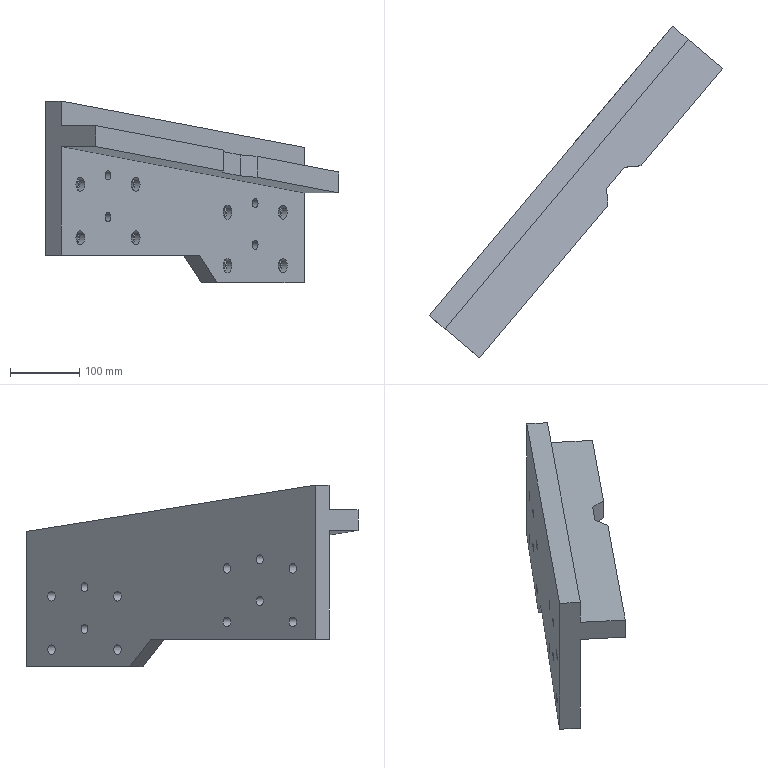Part | NX | features solid 2 | 1 solid | 44 faces | box 423.093 x 478.559 x 262.18 mm | volume 4319267 mm3 | plane 24 | cylinder 20 | commonest cylinder face diameters 14 x8 20 x8 13 x4
STEP:
#1=CARTESIAN_POINT('',(-445.328,317.148,-17.493));
#2=VERTEX_POINT('',#1);
#3=CARTESIAN_POINT('',(-327.504,457.565,-40.));
#4=VERTEX_POINT('',#3);
#5=CARTESIAN_POINT('',(-249.072,551.037,-54.982));
#6=DIRECTION('',(-0.638,-0.7603,0.1219));
#7=VECTOR('',#6,1000.);
#8=LINE('',#5,#7);
#9=EDGE_CURVE('',#2,#4,#8,.F.);
#10=ORIENTED_EDGE('',*,*,#9,.F.);
#11=CARTESIAN_POINT('',(-445.328,317.148,-47.719));
#12=VERTEX_POINT('',#11);
#13=CARTESIAN_POINT('',(-445.328,317.148,-55.974));
#14=DIRECTION('',(0.,0.,-1.));
#15=VECTOR('',#14,1000.);
#16=LINE('',#13,#15);
#17=EDGE_CURVE('',#2,#12,#16,.T.);
#18=ORIENTED_EDGE('',*,*,#17,.T.);
#19=CARTESIAN_POINT('',(-327.504,457.565,-70.225));
#20=VERTEX_POINT('',#19);
#21=CARTESIAN_POINT('',(-281.119,512.845,-79.086));
#22=DIRECTION('',(0.638,0.7603,-0.1219));
#23=VECTOR('',#22,1000.);
#24=LINE('',#21,#23);
#25=EDGE_CURVE('',#12,#20,#24,.T.);
#26=ORIENTED_EDGE('',*,*,#25,.T.);
#27=CARTESIAN_POINT('',(-327.504,457.565,-15.974));
#28=DIRECTION('',(0.,0.,1.));
#29=VECTOR('',#28,1000.);
#30=LINE('',#27,#29);
#31=EDGE_CURVE('',#4,#20,#30,.F.);
#32=ORIENTED_EDGE('',*,*,#31,.F.);
#33=EDGE_LOOP('',(#10,#18,#26,#32));
#34=FACE_BOUND('',#33,.T.);
#35=CARTESIAN_POINT('',(-279.295,515.019,-55.974));
#36=DIRECTION('',(-0.766,0.6428,0.));
#37=DIRECTION('',(-0.6428,-0.766,0.));
#38=AXIS2_PLACEMENT_3D('',#35,#36,#37);
#39=PLANE('',#38);
#40=ADVANCED_FACE('',(#34),#39,.F.);
#41=CARTESIAN_POINT('',(-494.284,359.927,-98.));
#42=VERTEX_POINT('',#41);
#43=CARTESIAN_POINT('',(-487.856,367.587,-98.));
#44=DIRECTION('',(-0.766,0.6428,0.));
#45=DIRECTION('',(-0.6428,-0.766,0.));
#46=AXIS2_PLACEMENT_3D('',#43,#44,#45);
#47=CIRCLE('',#46,10.);
#48=EDGE_CURVE('',#42,#42,#47,.F.);
#49=ORIENTED_EDGE('',*,*,#48,.F.);
#50=EDGE_LOOP('',(#49));
#51=FACE_BOUND('',#50,.T.);
#52=CARTESIAN_POINT('',(-494.284,359.927,-175.));
#53=VERTEX_POINT('',#52);
#54=CARTESIAN_POINT('',(-487.856,367.587,-175.));
#55=DIRECTION('',(-0.766,0.6428,0.));
#56=DIRECTION('',(-0.6428,-0.766,0.));
#57=AXIS2_PLACEMENT_3D('',#54,#55,#56);
#58=CIRCLE('',#57,10.);
#59=EDGE_CURVE('',#53,#53,#58,.F.);
#60=ORIENTED_EDGE('',*,*,#59,.F.);
#61=EDGE_LOOP('',(#60));
#62=FACE_BOUND('',#61,.T.);
#63=CARTESIAN_POINT('',(-626.698,202.121,-135.));
#64=VERTEX_POINT('',#63);
#65=CARTESIAN_POINT('',(-620.271,209.782,-135.));
#66=DIRECTION('',(-0.766,0.6428,0.));
#67=DIRECTION('',(-0.6428,-0.766,0.));
#68=AXIS2_PLACEMENT_3D('',#65,#66,#67);
#69=CIRCLE('',#68,10.);
#70=EDGE_CURVE('',#64,#64,#69,.F.);
#71=ORIENTED_EDGE('',*,*,#70,.F.);
#72=EDGE_LOOP('',(#71));
#73=FACE_BOUND('',#72,.T.);
#74=CARTESIAN_POINT('',(-706.404,107.132,-58.));
#75=VERTEX_POINT('',#74);
#76=CARTESIAN_POINT('',(-699.976,114.792,-58.));
#77=DIRECTION('',(-0.766,0.6428,0.));
#78=DIRECTION('',(-0.6428,-0.766,0.));
#79=AXIS2_PLACEMENT_3D('',#76,#77,#78);
#80=CIRCLE('',#79,10.);
#81=EDGE_CURVE('',#75,#75,#80,.F.);
#82=ORIENTED_EDGE('',*,*,#81,.F.);
#83=EDGE_LOOP('',(#82));
#84=FACE_BOUND('',#83,.T.);
#85=CARTESIAN_POINT('',(-727.616,81.852,-160.));
#86=VERTEX_POINT('',#85);
#87=CARTESIAN_POINT('',(-528.352,319.326,-160.));
#88=VERTEX_POINT('',#87);
#89=CARTESIAN_POINT('',(-727.616,81.852,-160.));
#90=DIRECTION('',(0.6428,0.766,0.));
#91=VECTOR('',#90,1000.);
#92=LINE('',#89,#91);
#93=EDGE_CURVE('',#86,#88,#92,.T.);
#94=ORIENTED_EDGE('',*,*,#93,.T.);
#95=CARTESIAN_POINT('',(-502.64,349.968,-200.));
#96=VERTEX_POINT('',#95);
#97=CARTESIAN_POINT('',(-475.009,382.898,-242.987));
#98=DIRECTION('',(0.4545,0.5417,-0.7071));
#99=VECTOR('',#98,1000.);
#100=LINE('',#97,#99);
#101=EDGE_CURVE('',#88,#96,#100,.T.);
#102=ORIENTED_EDGE('',*,*,#101,.T.);
#103=CARTESIAN_POINT('',(-377.297,499.347,-200.));
#104=VERTEX_POINT('',#103);
#105=CARTESIAN_POINT('',(-329.088,556.8,-200.));
#106=DIRECTION('',(-0.6428,-0.766,0.));
#107=VECTOR('',#106,1000.);
#108=LINE('',#105,#107);
#109=EDGE_CURVE('',#96,#104,#108,.F.);
#110=ORIENTED_EDGE('',*,*,#109,.T.);
#111=CARTESIAN_POINT('',(-377.297,499.347,-70.225));
#112=VERTEX_POINT('',#111);
#113=CARTESIAN_POINT('',(-377.297,499.347,-15.974));
#114=DIRECTION('',(0.,0.,1.));
#115=VECTOR('',#114,1000.);
#116=LINE('',#113,#115);
#117=EDGE_CURVE('',#112,#104,#116,.F.);
#118=ORIENTED_EDGE('',*,*,#117,.F.);
#119=CARTESIAN_POINT('',(-727.616,81.852,-3.308));
#120=VERTEX_POINT('',#119);
#121=CARTESIAN_POINT('',(-553.34,289.547,-36.598));
#122=DIRECTION('',(0.638,0.7603,-0.1219));
#123=VECTOR('',#122,1000.);
#124=LINE('',#121,#123);
#125=EDGE_CURVE('',#120,#112,#124,.T.);
#126=ORIENTED_EDGE('',*,*,#125,.F.);
#127=CARTESIAN_POINT('',(-727.616,81.852,-70.036));
#128=DIRECTION('',(0.,0.,-1.));
#129=VECTOR('',#128,1000.);
#130=LINE('',#127,#129);
#131=EDGE_CURVE('',#86,#120,#130,.F.);
#132=ORIENTED_EDGE('',*,*,#131,.F.);
#133=EDGE_LOOP('',(#94,#102,#110,#118,#126,#132));
#134=FACE_BOUND('',#133,.T.);
#135=CARTESIAN_POINT('',(-664.302,157.308,-105.));
#136=VERTEX_POINT('',#135);
#137=CARTESIAN_POINT('',(-660.123,162.287,-105.));
#138=DIRECTION('',(-0.766,0.6428,0.));
#139=DIRECTION('',(-0.6428,-0.766,0.));
#140=AXIS2_PLACEMENT_3D('',#137,#138,#139);
#141=CIRCLE('',#140,6.5);
#142=EDGE_CURVE('',#136,#136,#141,.T.);
#143=ORIENTED_EDGE('',*,*,#142,.T.);
#144=EDGE_LOOP('',(#143));
#145=FACE_BOUND('',#144,.T.);
#146=CARTESIAN_POINT('',(-664.302,157.308,-45.));
#147=VERTEX_POINT('',#146);
#148=CARTESIAN_POINT('',(-660.123,162.287,-45.));
#149=DIRECTION('',(-0.766,0.6428,0.));
#150=DIRECTION('',(-0.6428,-0.766,0.));
#151=AXIS2_PLACEMENT_3D('',#148,#149,#150);
#152=CIRCLE('',#151,6.5);
#153=EDGE_CURVE('',#147,#147,#152,.T.);
#154=ORIENTED_EDGE('',*,*,#153,.T.);
#155=EDGE_LOOP('',(#154));
#156=FACE_BOUND('',#155,.T.);
#157=CARTESIAN_POINT('',(-452.182,410.102,-145.));
#158=VERTEX_POINT('',#157);
#159=CARTESIAN_POINT('',(-448.003,415.082,-145.));
#160=DIRECTION('',(-0.766,0.6428,0.));
#161=DIRECTION('',(-0.6428,-0.766,0.));
#162=AXIS2_PLACEMENT_3D('',#159,#160,#161);
#163=CIRCLE('',#162,6.5);
#164=EDGE_CURVE('',#158,#158,#163,.T.);
#165=ORIENTED_EDGE('',*,*,#164,.T.);
#166=EDGE_LOOP('',(#165));
#167=FACE_BOUND('',#166,.T.);
#168=CARTESIAN_POINT('',(-452.182,410.102,-85.));
#169=VERTEX_POINT('',#168);
#170=CARTESIAN_POINT('',(-448.003,415.082,-85.));
#171=DIRECTION('',(-0.766,0.6428,0.));
#172=DIRECTION('',(-0.6428,-0.766,0.));
#173=AXIS2_PLACEMENT_3D('',#170,#171,#172);
#174=CIRCLE('',#173,6.5);
#175=EDGE_CURVE('',#169,#169,#174,.T.);
#176=ORIENTED_EDGE('',*,*,#175,.T.);
#177=EDGE_LOOP('',(#176));
#178=FACE_BOUND('',#177,.T.);
#179=CARTESIAN_POINT('',(-706.404,107.132,-135.));
#180=VERTEX_POINT('',#179);
#181=CARTESIAN_POINT('',(-699.976,114.792,-135.));
#182=DIRECTION('',(-0.766,0.6428,0.));
#183=DIRECTION('',(-0.6428,-0.766,0.));
#184=AXIS2_PLACEMENT_3D('',#181,#182,#183);
#185=CIRCLE('',#184,10.);
#186=EDGE_CURVE('',#180,#180,#185,.F.);
#187=ORIENTED_EDGE('',*,*,#186,.F.);
#188=EDGE_LOOP('',(#187));
#189=FACE_BOUND('',#188,.T.);
#190=CARTESIAN_POINT('',(-626.698,202.121,-58.));
#191=VERTEX_POINT('',#190);
#192=CARTESIAN_POINT('',(-620.271,209.782,-58.));
#193=DIRECTION('',(-0.766,0.6428,0.));
#194=DIRECTION('',(-0.6428,-0.766,0.));
#195=AXIS2_PLACEMENT_3D('',#192,#193,#194);
#196=CIRCLE('',#195,10.);
#197=EDGE_CURVE('',#191,#191,#196,.F.);
#198=ORIENTED_EDGE('',*,*,#197,.F.);
#199=EDGE_LOOP('',(#198));
#200=FACE_BOUND('',#199,.T.);
#201=CARTESIAN_POINT('',(-414.579,454.916,-175.));
#202=VERTEX_POINT('',#201);
#203=CARTESIAN_POINT('',(-408.151,462.577,-175.));
#204=DIRECTION('',(-0.766,0.6428,0.));
#205=DIRECTION('',(-0.6428,-0.766,0.));
#206=AXIS2_PLACEMENT_3D('',#203,#204,#205);
#207=CIRCLE('',#206,10.);
#208=EDGE_CURVE('',#202,#202,#207,.F.);
#209=ORIENTED_EDGE('',*,*,#208,.F.);
#210=EDGE_LOOP('',(#209));
#211=FACE_BOUND('',#210,.T.);
#212=CARTESIAN_POINT('',(-414.579,454.916,-98.));
#213=VERTEX_POINT('',#212);
#214=CARTESIAN_POINT('',(-408.151,462.577,-98.));
#215=DIRECTION('',(-0.766,0.6428,0.));
#216=DIRECTION('',(-0.6428,-0.766,0.));
#217=AXIS2_PLACEMENT_3D('',#214,#215,#216);
#218=CIRCLE('',#217,10.);
#219=EDGE_CURVE('',#213,#213,#218,.F.);
#220=ORIENTED_EDGE('',*,*,#219,.F.);
#221=EDGE_LOOP('',(#220));
#222=FACE_BOUND('',#221,.T.);
#223=CARTESIAN_POINT('',(-329.088,556.8,-15.974));
#224=DIRECTION('',(-0.766,0.6428,0.));
#225=DIRECTION('',(-0.6428,-0.766,0.));
#226=AXIS2_PLACEMENT_3D('',#223,#224,#225);
#227=PLANE('',#226);
#228=ADVANCED_FACE('',(#51,#62,#73,#84,#134,#145,#156,#167,#178,#189,#200,#211,#222),#227,.F.);
#229=CARTESIAN_POINT('',(-525.622,369.252,-200.));
#230=VERTEX_POINT('',#229);
#231=CARTESIAN_POINT('',(-400.278,518.63,-200.));
#232=VERTEX_POINT('',#231);
#233=CARTESIAN_POINT('',(-352.069,576.084,-200.));
#234=DIRECTION('',(-0.6428,-0.766,0.));
#235=VECTOR('',#234,1000.);
#236=LINE('',#233,#235);
#237=EDGE_CURVE('',#230,#232,#236,.F.);
#238=ORIENTED_EDGE('',*,*,#237,.F.);
#239=CARTESIAN_POINT('',(-551.333,338.61,-160.));
#240=VERTEX_POINT('',#239);
#241=CARTESIAN_POINT('',(-551.333,338.61,-160.));
#242=DIRECTION('',(-0.4545,-0.5417,0.7071));
#243=VECTOR('',#242,1000.);
#244=LINE('',#241,#243);
#245=EDGE_CURVE('',#230,#240,#244,.T.);
#246=ORIENTED_EDGE('',*,*,#245,.T.);
#247=CARTESIAN_POINT('',(-750.597,101.136,-160.));
#248=VERTEX_POINT('',#247);
#249=CARTESIAN_POINT('',(-750.597,101.136,-160.));
#250=DIRECTION('',(0.6428,0.766,0.));
#251=VECTOR('',#250,1000.);
#252=LINE('',#249,#251);
#253=EDGE_CURVE('',#248,#240,#252,.T.);
#254=ORIENTED_EDGE('',*,*,#253,.F.);
#255=CARTESIAN_POINT('',(-750.597,101.136,62.18));
#256=VERTEX_POINT('',#255);
#257=CARTESIAN_POINT('',(-750.597,101.136,-15.974));
#258=DIRECTION('',(0.,0.,1.));
#259=VECTOR('',#258,1000.);
#260=LINE('',#257,#259);
#261=EDGE_CURVE('',#256,#248,#260,.F.);
#262=ORIENTED_EDGE('',*,*,#261,.F.);
#263=CARTESIAN_POINT('',(-400.278,518.63,-4.737));
#264=VERTEX_POINT('',#263);
#265=CARTESIAN_POINT('',(-319.104,615.369,-20.243));
#266=DIRECTION('',(-0.638,-0.7603,0.1219));
#267=VECTOR('',#266,1000.);
#268=LINE('',#265,#267);
#269=EDGE_CURVE('',#256,#264,#268,.F.);
#270=ORIENTED_EDGE('',*,*,#269,.T.);
#271=CARTESIAN_POINT('',(-400.278,518.63,-15.974));
#272=DIRECTION('',(0.,0.,1.));
#273=VECTOR('',#272,1000.);
#274=LINE('',#271,#273);
#275=EDGE_CURVE('',#264,#232,#274,.F.);
#276=ORIENTED_EDGE('',*,*,#275,.T.);
#277=EDGE_LOOP('',(#238,#246,#254,#262,#270,#276));
#278=FACE_BOUND('',#277,.T.);
#279=CARTESIAN_POINT('',(-647.751,223.703,-58.));
#280=VERTEX_POINT('',#279);
#281=CARTESIAN_POINT('',(-643.252,229.065,-58.));
#282=DIRECTION('',(-0.766,0.6428,0.));
#283=DIRECTION('',(-0.6428,-0.766,0.));
#284=AXIS2_PLACEMENT_3D('',#281,#282,#283);
#285=CIRCLE('',#284,7.);
#286=EDGE_CURVE('',#280,#280,#285,.F.);
#287=ORIENTED_EDGE('',*,*,#286,.T.);
#288=EDGE_LOOP('',(#287));
#289=FACE_BOUND('',#288,.T.);
#290=CARTESIAN_POINT('',(-687.283,176.591,-45.));
#291=VERTEX_POINT('',#290);
#292=CARTESIAN_POINT('',(-683.105,181.571,-45.));
#293=DIRECTION('',(-0.766,0.6428,0.));
#294=DIRECTION('',(-0.6428,-0.766,0.));
#295=AXIS2_PLACEMENT_3D('',#292,#293,#294);
#296=CIRCLE('',#295,6.5);
#297=EDGE_CURVE('',#291,#291,#296,.T.);
#298=ORIENTED_EDGE('',*,*,#297,.F.);
#299=EDGE_LOOP('',(#298));
#300=FACE_BOUND('',#299,.T.);
#301=CARTESIAN_POINT('',(-647.751,223.703,-135.));
#302=VERTEX_POINT('',#301);
#303=CARTESIAN_POINT('',(-643.252,229.065,-135.));
#304=DIRECTION('',(-0.766,0.6428,0.));
#305=DIRECTION('',(-0.6428,-0.766,0.));
#306=AXIS2_PLACEMENT_3D('',#303,#304,#305);
#307=CIRCLE('',#306,7.);
#308=EDGE_CURVE('',#302,#302,#307,.F.);
#309=ORIENTED_EDGE('',*,*,#308,.T.);
#310=EDGE_LOOP('',(#309));
#311=FACE_BOUND('',#310,.T.);
#312=CARTESIAN_POINT('',(-687.283,176.591,-105.));
#313=VERTEX_POINT('',#312);
#314=CARTESIAN_POINT('',(-683.105,181.571,-105.));
#315=DIRECTION('',(-0.766,0.6428,0.));
#316=DIRECTION('',(-0.6428,-0.766,0.));
#317=AXIS2_PLACEMENT_3D('',#314,#315,#316);
#318=CIRCLE('',#317,6.5);
#319=EDGE_CURVE('',#313,#313,#318,.T.);
#320=ORIENTED_EDGE('',*,*,#319,.F.);
#321=EDGE_LOOP('',(#320));
#322=FACE_BOUND('',#321,.T.);
#323=CARTESIAN_POINT('',(-727.457,128.714,-135.));
#324=VERTEX_POINT('',#323);
#325=CARTESIAN_POINT('',(-722.958,134.076,-135.));
#326=DIRECTION('',(-0.766,0.6428,0.));
#327=DIRECTION('',(-0.6428,-0.766,0.));
#328=AXIS2_PLACEMENT_3D('',#325,#326,#327);
#329=CIRCLE('',#328,7.);
#330=EDGE_CURVE('',#324,#324,#329,.F.);
#331=ORIENTED_EDGE('',*,*,#330,.T.);
#332=EDGE_LOOP('',(#331));
#333=FACE_BOUND('',#332,.T.);
#334=CARTESIAN_POINT('',(-727.457,128.714,-58.));
#335=VERTEX_POINT('',#334);
#336=CARTESIAN_POINT('',(-722.958,134.076,-58.));
#337=DIRECTION('',(-0.766,0.6428,0.));
#338=DIRECTION('',(-0.6428,-0.766,0.));
#339=AXIS2_PLACEMENT_3D('',#336,#337,#338);
#340=CIRCLE('',#339,7.);
#341=EDGE_CURVE('',#335,#335,#340,.F.);
#342=ORIENTED_EDGE('',*,*,#341,.T.);
#343=EDGE_LOOP('',(#342));
#344=FACE_BOUND('',#343,.T.);
#345=CARTESIAN_POINT('',(-435.631,476.498,-98.));
#346=VERTEX_POINT('',#345);
#347=CARTESIAN_POINT('',(-431.132,481.86,-98.));
#348=DIRECTION('',(-0.766,0.6428,0.));
#349=DIRECTION('',(-0.6428,-0.766,0.));
#350=AXIS2_PLACEMENT_3D('',#347,#348,#349);
#351=CIRCLE('',#350,7.);
#352=EDGE_CURVE('',#346,#346,#351,.F.);
#353=ORIENTED_EDGE('',*,*,#352,.T.);
#354=EDGE_LOOP('',(#353));
#355=FACE_BOUND('',#354,.T.);
#356=CARTESIAN_POINT('',(-475.163,429.386,-85.));
#357=VERTEX_POINT('',#356);
#358=CARTESIAN_POINT('',(-470.985,434.365,-85.));
#359=DIRECTION('',(-0.766,0.6428,0.));
#360=DIRECTION('',(-0.6428,-0.766,0.));
#361=AXIS2_PLACEMENT_3D('',#358,#359,#360);
#362=CIRCLE('',#361,6.5);
#363=EDGE_CURVE('',#357,#357,#362,.T.);
#364=ORIENTED_EDGE('',*,*,#363,.F.);
#365=EDGE_LOOP('',(#364));
#366=FACE_BOUND('',#365,.T.);
#367=CARTESIAN_POINT('',(-435.631,476.498,-175.));
#368=VERTEX_POINT('',#367);
#369=CARTESIAN_POINT('',(-431.132,481.86,-175.));
#370=DIRECTION('',(-0.766,0.6428,0.));
#371=DIRECTION('',(-0.6428,-0.766,0.));
#372=AXIS2_PLACEMENT_3D('',#369,#370,#371);
#373=CIRCLE('',#372,7.);
#374=EDGE_CURVE('',#368,#368,#373,.F.);
#375=ORIENTED_EDGE('',*,*,#374,.T.);
#376=EDGE_LOOP('',(#375));
#377=FACE_BOUND('',#376,.T.);
#378=CARTESIAN_POINT('',(-475.163,429.386,-145.));
#379=VERTEX_POINT('',#378);
#380=CARTESIAN_POINT('',(-470.985,434.365,-145.));
#381=DIRECTION('',(-0.766,0.6428,0.));
#382=DIRECTION('',(-0.6428,-0.766,0.));
#383=AXIS2_PLACEMENT_3D('',#380,#381,#382);
#384=CIRCLE('',#383,6.5);
#385=EDGE_CURVE('',#379,#379,#384,.T.);
#386=ORIENTED_EDGE('',*,*,#385,.F.);
#387=EDGE_LOOP('',(#386));
#388=FACE_BOUND('',#387,.T.);
#389=CARTESIAN_POINT('',(-515.337,381.508,-175.));
#390=VERTEX_POINT('',#389);
#391=CARTESIAN_POINT('',(-510.838,386.871,-175.));
#392=DIRECTION('',(-0.766,0.6428,0.));
#393=DIRECTION('',(-0.6428,-0.766,0.));
#394=AXIS2_PLACEMENT_3D('',#391,#392,#393);
#395=CIRCLE('',#394,7.);
#396=EDGE_CURVE('',#390,#390,#395,.F.);
#397=ORIENTED_EDGE('',*,*,#396,.T.);
#398=EDGE_LOOP('',(#397));
#399=FACE_BOUND('',#398,.T.);
#400=CARTESIAN_POINT('',(-515.337,381.508,-98.));
#401=VERTEX_POINT('',#400);
#402=CARTESIAN_POINT('',(-510.838,386.871,-98.));
#403=DIRECTION('',(-0.766,0.6428,0.));
#404=DIRECTION('',(-0.6428,-0.766,0.));
#405=AXIS2_PLACEMENT_3D('',#402,#403,#404);
#406=CIRCLE('',#405,7.);
#407=EDGE_CURVE('',#401,#401,#406,.F.);
#408=ORIENTED_EDGE('',*,*,#407,.T.);
#409=EDGE_LOOP('',(#408));
#410=FACE_BOUND('',#409,.T.);
#411=CARTESIAN_POINT('',(-352.069,576.084,-15.974));
#412=DIRECTION('',(-0.766,0.6428,0.));
#413=DIRECTION('',(-0.6428,-0.766,0.));
#414=AXIS2_PLACEMENT_3D('',#411,#412,#413);
#415=PLANE('',#414);
#416=ADVANCED_FACE('',(#278,#289,#300,#311,#322,#333,#344,#355,#366,#377,#388,#399,#410),#415,.T.);
#417=ORIENTED_EDGE('',*,*,#25,.F.);
#418=CARTESIAN_POINT('',(-469.331,315.048,-45.627));
#419=VERTEX_POINT('',#418);
#420=CARTESIAN_POINT('',(-555.051,307.548,-38.156));
#421=DIRECTION('',(-0.9925,-0.08683,0.0865));
#422=VECTOR('',#421,1000.);
#423=LINE('',#420,#422);
#424=EDGE_CURVE('',#12,#419,#423,.T.);
#425=ORIENTED_EDGE('',*,*,#424,.T.);
#426=CARTESIAN_POINT('',(-495.043,284.406,-40.715));
#427=VERTEX_POINT('',#426);
#428=CARTESIAN_POINT('',(-516.599,258.717,-36.598));
#429=DIRECTION('',(0.638,0.7603,-0.1219));
#430=VECTOR('',#429,1000.);
#431=LINE('',#428,#430);
#432=EDGE_CURVE('',#427,#419,#431,.T.);
#433=ORIENTED_EDGE('',*,*,#432,.F.);
#434=CARTESIAN_POINT('',(-492.943,260.403,-38.623));
#435=VERTEX_POINT('',#434);
#436=CARTESIAN_POINT('',(-495.895,294.14,-41.564));
#437=DIRECTION('',(0.08683,-0.9925,0.0865));
#438=VECTOR('',#437,1000.);
#439=LINE('',#436,#438);
#440=EDGE_CURVE('',#427,#435,#439,.T.);
#441=ORIENTED_EDGE('',*,*,#440,.T.);
#442=CARTESIAN_POINT('',(-677.823,40.071,-3.308));
#443=VERTEX_POINT('',#442);
#444=CARTESIAN_POINT('',(-281.119,512.845,-79.086));
#445=DIRECTION('',(0.638,0.7603,-0.1219));
#446=VECTOR('',#445,1000.);
#447=LINE('',#444,#446);
#448=EDGE_CURVE('',#443,#435,#447,.T.);
#449=ORIENTED_EDGE('',*,*,#448,.F.);
#450=CARTESIAN_POINT('',(-727.616,81.852,-3.308));
#451=DIRECTION('',(0.766,-0.6428,0.));
#452=VECTOR('',#451,1000.);
#453=LINE('',#450,#452);
#454=EDGE_CURVE('',#443,#120,#453,.F.);
#455=ORIENTED_EDGE('',*,*,#454,.T.);
#456=ORIENTED_EDGE('',*,*,#125,.T.);
#457=CARTESIAN_POINT('',(-377.297,499.347,-70.225));
#458=DIRECTION('',(0.766,-0.6428,0.));
#459=VECTOR('',#458,1000.);
#460=LINE('',#457,#459);
#461=EDGE_CURVE('',#20,#112,#460,.F.);
#462=ORIENTED_EDGE('',*,*,#461,.F.);
#463=EDGE_LOOP('',(#417,#425,#433,#441,#449,#455,#456,#462));
#464=FACE_BOUND('',#463,.T.);
#465=CARTESIAN_POINT('',(-553.34,289.547,-36.598));
#466=DIRECTION('',(0.07834,0.09336,0.9925));
#467=DIRECTION('',(0.638,0.7603,-0.1219));
#468=AXIS2_PLACEMENT_3D('',#465,#466,#467);
#469=PLANE('',#468);
#470=ADVANCED_FACE('',(#464),#469,.F.);
#471=CARTESIAN_POINT('',(-727.616,81.852,26.918));
#472=VERTEX_POINT('',#471);
#473=CARTESIAN_POINT('',(-377.297,499.347,-40.));
#474=VERTEX_POINT('',#473);
#475=CARTESIAN_POINT('',(-298.865,592.818,-54.982));
#476=DIRECTION('',(-0.638,-0.7603,0.1219));
#477=VECTOR('',#476,1000.);
#478=LINE('',#475,#477);
#479=EDGE_CURVE('',#472,#474,#478,.F.);
#480=ORIENTED_EDGE('',*,*,#479,.T.);
#481=CARTESIAN_POINT('',(-377.297,499.347,-4.737));
#482=VERTEX_POINT('',#481);
#483=CARTESIAN_POINT('',(-377.297,499.347,-15.974));
#484=DIRECTION('',(0.,0.,1.));
#485=VECTOR('',#484,1000.);
#486=LINE('',#483,#485);
#487=EDGE_CURVE('',#482,#474,#486,.F.);
#488=ORIENTED_EDGE('',*,*,#487,.F.);
#489=CARTESIAN_POINT('',(-727.616,81.852,62.18));
#490=VERTEX_POINT('',#489);
#491=CARTESIAN_POINT('',(-296.123,596.086,-20.243));
#492=DIRECTION('',(-0.638,-0.7603,0.1219));
#493=VECTOR('',#492,1000.);
#494=LINE('',#491,#493);
#495=EDGE_CURVE('',#490,#482,#494,.F.);
#496=ORIENTED_EDGE('',*,*,#495,.F.);
#497=CARTESIAN_POINT('',(-727.616,81.852,-15.974));
#498=DIRECTION('',(0.,0.,1.));
#499=VECTOR('',#498,1000.);
#500=LINE('',#497,#499);
#501=EDGE_CURVE('',#490,#472,#500,.F.);
#502=ORIENTED_EDGE('',*,*,#501,.T.);
#503=EDGE_LOOP('',(#480,#488,#496,#502));
#504=FACE_BOUND('',#503,.T.);
#505=CARTESIAN_POINT('',(-329.088,556.8,-15.974));
#506=DIRECTION('',(-0.766,0.6428,0.));
#507=DIRECTION('',(-0.6428,-0.766,0.));
#508=AXIS2_PLACEMENT_3D('',#505,#506,#507);
#509=PLANE('',#508);
#510=ADVANCED_FACE('',(#504),#509,.F.);
#511=ORIENTED_EDGE('',*,*,#495,.T.);
#512=CARTESIAN_POINT('',(-377.297,499.347,-4.737));
#513=DIRECTION('',(-0.766,0.6428,0.));
#514=VECTOR('',#513,1000.);
#515=LINE('',#512,#514);
#516=EDGE_CURVE('',#482,#264,#515,.T.);
#517=ORIENTED_EDGE('',*,*,#516,.T.);
#518=ORIENTED_EDGE('',*,*,#269,.F.);
#519=CARTESIAN_POINT('',(-727.616,81.852,62.18));
#520=DIRECTION('',(-0.766,0.6428,0.));
#521=VECTOR('',#520,1000.);
#522=LINE('',#519,#521);
#523=EDGE_CURVE('',#490,#256,#522,.T.);
#524=ORIENTED_EDGE('',*,*,#523,.F.);
#525=EDGE_LOOP('',(#511,#517,#518,#524));
#526=FACE_BOUND('',#525,.T.);
#527=CARTESIAN_POINT('',(-296.123,596.086,-20.243));
#528=DIRECTION('',(0.07834,0.09336,0.9925));
#529=DIRECTION('',(0.,-0.9956,0.09365));
#530=AXIS2_PLACEMENT_3D('',#527,#528,#529);
#531=PLANE('',#530);
#532=ADVANCED_FACE('',(#526),#531,.T.);
#533=ORIENTED_EDGE('',*,*,#109,.F.);
#534=CARTESIAN_POINT('',(-525.622,369.252,-200.));
#535=DIRECTION('',(0.766,-0.6428,0.));
#536=VECTOR('',#535,1000.);
#537=LINE('',#534,#536);
#538=EDGE_CURVE('',#230,#96,#537,.T.);
#539=ORIENTED_EDGE('',*,*,#538,.F.);
#540=ORIENTED_EDGE('',*,*,#237,.T.);
#541=CARTESIAN_POINT('',(-400.278,518.63,-200.));
#542=DIRECTION('',(-0.766,0.6428,0.));
#543=VECTOR('',#542,1000.);
#544=LINE('',#541,#543);
#545=EDGE_CURVE('',#104,#232,#544,.T.);
#546=ORIENTED_EDGE('',*,*,#545,.F.);
#547=EDGE_LOOP('',(#533,#539,#540,#546));
#548=FACE_BOUND('',#547,.T.);
#549=CARTESIAN_POINT('',(-470.985,434.365,-200.));
#550=DIRECTION('',(0.,0.,-1.));
#551=DIRECTION('',(-0.766,0.6428,0.));
#552=AXIS2_PLACEMENT_3D('',#549,#550,#551);
#553=PLANE('',#552);
#554=ADVANCED_FACE('',(#548),#553,.T.);
#555=ORIENTED_EDGE('',*,*,#461,.T.);
#556=ORIENTED_EDGE('',*,*,#117,.T.);
#557=ORIENTED_EDGE('',*,*,#545,.T.);
#558=ORIENTED_EDGE('',*,*,#275,.F.);
#559=ORIENTED_EDGE('',*,*,#516,.F.);
#560=ORIENTED_EDGE('',*,*,#487,.T.);
#561=CARTESIAN_POINT('',(-377.297,499.347,-40.));
#562=DIRECTION('',(0.766,-0.6428,0.));
#563=VECTOR('',#562,1000.);
#564=LINE('',#561,#563);
#565=EDGE_CURVE('',#474,#4,#564,.T.);
#566=ORIENTED_EDGE('',*,*,#565,.T.);
#567=ORIENTED_EDGE('',*,*,#31,.T.);
#568=EDGE_LOOP('',(#555,#556,#557,#558,#559,#560,#566,#567));
#569=FACE_BOUND('',#568,.T.);
#570=CARTESIAN_POINT('',(-377.297,499.347,-15.974));
#571=DIRECTION('',(0.6428,0.766,0.));
#572=DIRECTION('',(0.,0.,-1.));
#573=AXIS2_PLACEMENT_3D('',#570,#571,#572);
#574=PLANE('',#573);
#575=ADVANCED_FACE('',(#569),#574,.T.);
#576=ORIENTED_EDGE('',*,*,#448,.T.);
#577=CARTESIAN_POINT('',(-492.943,260.403,-8.398));
#578=VERTEX_POINT('',#577);
#579=CARTESIAN_POINT('',(-492.943,260.403,-55.974));
#580=DIRECTION('',(0.,0.,1.));
#581=VECTOR('',#580,1000.);
#582=LINE('',#579,#581);
#583=EDGE_CURVE('',#435,#578,#582,.T.);
#584=ORIENTED_EDGE('',*,*,#583,.T.);
#585=CARTESIAN_POINT('',(-677.823,40.071,26.918));
#586=VERTEX_POINT('',#585);
#587=CARTESIAN_POINT('',(-249.072,551.037,-54.982));
#588=DIRECTION('',(-0.638,-0.7603,0.1219));
#589=VECTOR('',#588,1000.);
#590=LINE('',#587,#589);
#591=EDGE_CURVE('',#586,#578,#590,.F.);
#592=ORIENTED_EDGE('',*,*,#591,.F.);
#593=CARTESIAN_POINT('',(-677.823,40.071,-55.974));
#594=DIRECTION('',(0.,0.,1.));
#595=VECTOR('',#594,1000.);
#596=LINE('',#593,#595);
#597=EDGE_CURVE('',#586,#443,#596,.F.);
#598=ORIENTED_EDGE('',*,*,#597,.T.);
#599=EDGE_LOOP('',(#576,#584,#592,#598));
#600=FACE_BOUND('',#599,.T.);
#601=CARTESIAN_POINT('',(-279.295,515.019,-55.974));
#602=DIRECTION('',(-0.766,0.6428,0.));
#603=DIRECTION('',(-0.6428,-0.766,0.));
#604=AXIS2_PLACEMENT_3D('',#601,#602,#603);
#605=PLANE('',#604);
#606=ADVANCED_FACE('',(#600),#605,.F.);
#607=CARTESIAN_POINT('',(-469.331,315.048,-15.401));
#608=VERTEX_POINT('',#607);
#609=CARTESIAN_POINT('',(-495.043,284.406,-10.49));
#610=VERTEX_POINT('',#609);
#611=CARTESIAN_POINT('',(-262.123,561.989,-54.982));
#612=DIRECTION('',(0.638,0.7603,-0.1219));
#613=VECTOR('',#612,1000.);
#614=LINE('',#611,#613);
#615=EDGE_CURVE('',#608,#610,#614,.F.);
#616=ORIENTED_EDGE('',*,*,#615,.F.);
#617=CARTESIAN_POINT('',(-274.091,332.129,-32.417));
#618=DIRECTION('',(-0.9925,-0.08683,0.0865));
#619=VECTOR('',#618,1000.);
#620=LINE('',#617,#619);
#621=EDGE_CURVE('',#608,#2,#620,.F.);
#622=ORIENTED_EDGE('',*,*,#621,.T.);
#623=ORIENTED_EDGE('',*,*,#9,.T.);
#624=ORIENTED_EDGE('',*,*,#565,.F.);
#625=ORIENTED_EDGE('',*,*,#479,.F.);
#626=CARTESIAN_POINT('',(-727.616,81.852,26.918));
#627=DIRECTION('',(0.766,-0.6428,0.));
#628=VECTOR('',#627,1000.);
#629=LINE('',#626,#628);
#630=EDGE_CURVE('',#472,#586,#629,.T.);
#631=ORIENTED_EDGE('',*,*,#630,.T.);
#632=ORIENTED_EDGE('',*,*,#591,.T.);
#633=CARTESIAN_POINT('',(-520.475,575.099,-35.825));
#634=DIRECTION('',(0.08683,-0.9925,0.0865));
#635=VECTOR('',#634,1000.);
#636=LINE('',#633,#635);
#637=EDGE_CURVE('',#578,#610,#636,.F.);
#638=ORIENTED_EDGE('',*,*,#637,.T.);
#639=EDGE_LOOP('',(#616,#622,#623,#624,#625,#631,#632,#638));
#640=FACE_BOUND('',#639,.T.);
#641=CARTESIAN_POINT('',(-298.865,592.818,-54.982));
#642=DIRECTION('',(0.07834,0.09336,0.9925));
#643=DIRECTION('',(0.,-0.9956,0.09365));
#644=AXIS2_PLACEMENT_3D('',#641,#642,#643);
#645=PLANE('',#644);
#646=ADVANCED_FACE('',(#640),#645,.T.);
#647=CARTESIAN_POINT('',(-500.016,368.653,-175.));
#648=VERTEX_POINT('',#647);
#649=CARTESIAN_POINT('',(-495.517,374.015,-175.));
#650=DIRECTION('',(-0.766,0.6428,0.));
#651=DIRECTION('',(-0.6428,-0.766,0.));
#652=AXIS2_PLACEMENT_3D('',#649,#650,#651);
#653=CIRCLE('',#652,7.);
#654=EDGE_CURVE('',#648,#648,#653,.T.);
#655=ORIENTED_EDGE('',*,*,#654,.F.);
#656=EDGE_LOOP('',(#655));
#657=FACE_BOUND('',#656,.T.);
#658=ORIENTED_EDGE('',*,*,#396,.F.);
#659=EDGE_LOOP('',(#658));
#660=FACE_BOUND('',#659,.T.);
#661=CARTESIAN_POINT('',(-587.442,451.149,-175.));
#662=DIRECTION('',(0.766,-0.6428,0.));
#663=DIRECTION('',(0.,0.,-1.));
#664=AXIS2_PLACEMENT_3D('',#661,#662,#663);
#665=CYLINDRICAL_SURFACE('',#664,7.);
#666=ADVANCED_FACE('',(#657,#660),#665,.F.);
#667=ORIENTED_EDGE('',*,*,#385,.T.);
#668=EDGE_LOOP('',(#667));
#669=FACE_BOUND('',#668,.T.);
#670=ORIENTED_EDGE('',*,*,#164,.F.);
#671=EDGE_LOOP('',(#670));
#672=FACE_BOUND('',#671,.T.);
#673=CARTESIAN_POINT('',(-547.589,498.644,-145.));
#674=DIRECTION('',(0.766,-0.6428,0.));
#675=DIRECTION('',(0.,0.,-1.));
#676=AXIS2_PLACEMENT_3D('',#673,#674,#675);
#677=CYLINDRICAL_SURFACE('',#676,6.5);
#678=ADVANCED_FACE('',(#669,#672),#677,.F.);
#679=CARTESIAN_POINT('',(-420.311,463.642,-175.));
#680=VERTEX_POINT('',#679);
#681=CARTESIAN_POINT('',(-415.811,469.004,-175.));
#682=DIRECTION('',(-0.766,0.6428,0.));
#683=DIRECTION('',(-0.6428,-0.766,0.));
#684=AXIS2_PLACEMENT_3D('',#681,#682,#683);
#685=CIRCLE('',#684,7.);
#686=EDGE_CURVE('',#680,#680,#685,.T.);
#687=ORIENTED_EDGE('',*,*,#686,.F.);
#688=EDGE_LOOP('',(#687));
#689=FACE_BOUND('',#688,.T.);
#690=ORIENTED_EDGE('',*,*,#374,.F.);
#691=EDGE_LOOP('',(#690));
#692=FACE_BOUND('',#691,.T.);
#693=CARTESIAN_POINT('',(-507.736,546.139,-175.));
#694=DIRECTION('',(0.766,-0.6428,0.));
#695=DIRECTION('',(0.,0.,-1.));
#696=AXIS2_PLACEMENT_3D('',#693,#694,#695);
#697=CYLINDRICAL_SURFACE('',#696,7.);
#698=ADVANCED_FACE('',(#689,#692),#697,.F.);
#699=CARTESIAN_POINT('',(-500.016,368.653,-98.));
#700=VERTEX_POINT('',#699);
#701=CARTESIAN_POINT('',(-495.517,374.015,-98.));
#702=DIRECTION('',(-0.766,0.6428,0.));
#703=DIRECTION('',(-0.6428,-0.766,0.));
#704=AXIS2_PLACEMENT_3D('',#701,#702,#703);
#705=CIRCLE('',#704,7.);
#706=EDGE_CURVE('',#700,#700,#705,.T.);
#707=ORIENTED_EDGE('',*,*,#706,.F.);
#708=EDGE_LOOP('',(#707));
#709=FACE_BOUND('',#708,.T.);
#710=ORIENTED_EDGE('',*,*,#407,.F.);
#711=EDGE_LOOP('',(#710));
#712=FACE_BOUND('',#711,.T.);
#713=CARTESIAN_POINT('',(-587.442,451.149,-98.));
#714=DIRECTION('',(0.766,-0.6428,0.));
#715=DIRECTION('',(0.,0.,-1.));
#716=AXIS2_PLACEMENT_3D('',#713,#714,#715);
#717=CYLINDRICAL_SURFACE('',#716,7.);
#718=ADVANCED_FACE('',(#709,#712),#717,.F.);
#719=ORIENTED_EDGE('',*,*,#363,.T.);
#720=EDGE_LOOP('',(#719));
#721=FACE_BOUND('',#720,.T.);
#722=ORIENTED_EDGE('',*,*,#175,.F.);
#723=EDGE_LOOP('',(#722));
#724=FACE_BOUND('',#723,.T.);
#725=CARTESIAN_POINT('',(-547.589,498.644,-85.));
#726=DIRECTION('',(0.766,-0.6428,0.));
#727=DIRECTION('',(0.,0.,-1.));
#728=AXIS2_PLACEMENT_3D('',#725,#726,#727);
#729=CYLINDRICAL_SURFACE('',#728,6.5);
#730=ADVANCED_FACE('',(#721,#724),#729,.F.);
#731=CARTESIAN_POINT('',(-420.311,463.642,-98.));
#732=VERTEX_POINT('',#731);
#733=CARTESIAN_POINT('',(-415.811,469.004,-98.));
#734=DIRECTION('',(-0.766,0.6428,0.));
#735=DIRECTION('',(-0.6428,-0.766,0.));
#736=AXIS2_PLACEMENT_3D('',#733,#734,#735);
#737=CIRCLE('',#736,7.);
#738=EDGE_CURVE('',#732,#732,#737,.T.);
#739=ORIENTED_EDGE('',*,*,#738,.F.);
#740=EDGE_LOOP('',(#739));
#741=FACE_BOUND('',#740,.T.);
#742=ORIENTED_EDGE('',*,*,#352,.F.);
#743=EDGE_LOOP('',(#742));
#744=FACE_BOUND('',#743,.T.);
#745=CARTESIAN_POINT('',(-507.736,546.139,-98.));
#746=DIRECTION('',(0.766,-0.6428,0.));
#747=DIRECTION('',(0.,0.,-1.));
#748=AXIS2_PLACEMENT_3D('',#745,#746,#747);
#749=CYLINDRICAL_SURFACE('',#748,7.);
#750=ADVANCED_FACE('',(#741,#744),#749,.F.);
#751=ORIENTED_EDGE('',*,*,#261,.T.);
#752=CARTESIAN_POINT('',(-750.597,101.136,-160.));
#753=DIRECTION('',(0.766,-0.6428,0.));
#754=VECTOR('',#753,1000.);
#755=LINE('',#752,#754);
#756=EDGE_CURVE('',#248,#86,#755,.T.);
#757=ORIENTED_EDGE('',*,*,#756,.T.);
#758=ORIENTED_EDGE('',*,*,#131,.T.);
#759=ORIENTED_EDGE('',*,*,#454,.F.);
#760=ORIENTED_EDGE('',*,*,#597,.F.);
#761=ORIENTED_EDGE('',*,*,#630,.F.);
#762=ORIENTED_EDGE('',*,*,#501,.F.);
#763=ORIENTED_EDGE('',*,*,#523,.T.);
#764=EDGE_LOOP('',(#751,#757,#758,#759,#760,#761,#762,#763));
#765=FACE_BOUND('',#764,.T.);
#766=CARTESIAN_POINT('',(-727.616,81.852,-70.036));
#767=DIRECTION('',(-0.6428,-0.766,0.));
#768=DIRECTION('',(0.,0.,-1.));
#769=AXIS2_PLACEMENT_3D('',#766,#767,#768);
#770=PLANE('',#769);
#771=ADVANCED_FACE('',(#765),#770,.T.);
#772=CARTESIAN_POINT('',(-712.136,115.858,-135.));
#773=VERTEX_POINT('',#772);
#774=CARTESIAN_POINT('',(-707.637,121.22,-135.));
#775=DIRECTION('',(-0.766,0.6428,0.));
#776=DIRECTION('',(-0.6428,-0.766,0.));
#777=AXIS2_PLACEMENT_3D('',#774,#775,#776);
#778=CIRCLE('',#777,7.);
#779=EDGE_CURVE('',#773,#773,#778,.T.);
#780=ORIENTED_EDGE('',*,*,#779,.F.);
#781=EDGE_LOOP('',(#780));
#782=FACE_BOUND('',#781,.T.);
#783=ORIENTED_EDGE('',*,*,#330,.F.);
#784=EDGE_LOOP('',(#783));
#785=FACE_BOUND('',#784,.T.);
#786=CARTESIAN_POINT('',(-799.562,198.355,-135.));
#787=DIRECTION('',(0.766,-0.6428,0.));
#788=DIRECTION('',(0.,0.,-1.));
#789=AXIS2_PLACEMENT_3D('',#786,#787,#788);
#790=CYLINDRICAL_SURFACE('',#789,7.);
#791=ADVANCED_FACE('',(#782,#785),#790,.F.);
#792=ORIENTED_EDGE('',*,*,#319,.T.);
#793=EDGE_LOOP('',(#792));
#794=FACE_BOUND('',#793,.T.);
#795=ORIENTED_EDGE('',*,*,#142,.F.);
#796=EDGE_LOOP('',(#795));
#797=FACE_BOUND('',#796,.T.);
#798=CARTESIAN_POINT('',(-759.709,245.849,-105.));
#799=DIRECTION('',(0.766,-0.6428,0.));
#800=DIRECTION('',(0.,0.,-1.));
#801=AXIS2_PLACEMENT_3D('',#798,#799,#800);
#802=CYLINDRICAL_SURFACE('',#801,6.5);
#803=ADVANCED_FACE('',(#794,#797),#802,.F.);
#804=CARTESIAN_POINT('',(-632.431,210.847,-135.));
#805=VERTEX_POINT('',#804);
#806=CARTESIAN_POINT('',(-627.931,216.21,-135.));
#807=DIRECTION('',(-0.766,0.6428,0.));
#808=DIRECTION('',(-0.6428,-0.766,0.));
#809=AXIS2_PLACEMENT_3D('',#806,#807,#808);
#810=CIRCLE('',#809,7.);
#811=EDGE_CURVE('',#805,#805,#810,.T.);
#812=ORIENTED_EDGE('',*,*,#811,.F.);
#813=EDGE_LOOP('',(#812));
#814=FACE_BOUND('',#813,.T.);
#815=ORIENTED_EDGE('',*,*,#308,.F.);
#816=EDGE_LOOP('',(#815));
#817=FACE_BOUND('',#816,.T.);
#818=CARTESIAN_POINT('',(-719.856,293.344,-135.));
#819=DIRECTION('',(0.766,-0.6428,0.));
#820=DIRECTION('',(0.,0.,-1.));
#821=AXIS2_PLACEMENT_3D('',#818,#819,#820);
#822=CYLINDRICAL_SURFACE('',#821,7.);
#823=ADVANCED_FACE('',(#814,#817),#822,.F.);
#824=CARTESIAN_POINT('',(-712.136,115.858,-58.));
#825=VERTEX_POINT('',#824);
#826=CARTESIAN_POINT('',(-707.637,121.22,-58.));
#827=DIRECTION('',(-0.766,0.6428,0.));
#828=DIRECTION('',(-0.6428,-0.766,0.));
#829=AXIS2_PLACEMENT_3D('',#826,#827,#828);
#830=CIRCLE('',#829,7.);
#831=EDGE_CURVE('',#825,#825,#830,.T.);
#832=ORIENTED_EDGE('',*,*,#831,.F.);
#833=EDGE_LOOP('',(#832));
#834=FACE_BOUND('',#833,.T.);
#835=ORIENTED_EDGE('',*,*,#341,.F.);
#836=EDGE_LOOP('',(#835));
#837=FACE_BOUND('',#836,.T.);
#838=CARTESIAN_POINT('',(-799.562,198.355,-58.));
#839=DIRECTION('',(0.766,-0.6428,0.));
#840=DIRECTION('',(0.,0.,-1.));
#841=AXIS2_PLACEMENT_3D('',#838,#839,#840);
#842=CYLINDRICAL_SURFACE('',#841,7.);
#843=ADVANCED_FACE('',(#834,#837),#842,.F.);
#844=ORIENTED_EDGE('',*,*,#297,.T.);
#845=EDGE_LOOP('',(#844));
#846=FACE_BOUND('',#845,.T.);
#847=ORIENTED_EDGE('',*,*,#153,.F.);
#848=EDGE_LOOP('',(#847));
#849=FACE_BOUND('',#848,.T.);
#850=CARTESIAN_POINT('',(-759.709,245.849,-45.));
#851=DIRECTION('',(0.766,-0.6428,0.));
#852=DIRECTION('',(0.,0.,-1.));
#853=AXIS2_PLACEMENT_3D('',#850,#851,#852);
#854=CYLINDRICAL_SURFACE('',#853,6.5);
#855=ADVANCED_FACE('',(#846,#849),#854,.F.);
#856=CARTESIAN_POINT('',(-632.431,210.847,-58.));
#857=VERTEX_POINT('',#856);
#858=CARTESIAN_POINT('',(-627.931,216.21,-58.));
#859=DIRECTION('',(-0.766,0.6428,0.));
#860=DIRECTION('',(-0.6428,-0.766,0.));
#861=AXIS2_PLACEMENT_3D('',#858,#859,#860);
#862=CIRCLE('',#861,7.);
#863=EDGE_CURVE('',#857,#857,#862,.T.);
#864=ORIENTED_EDGE('',*,*,#863,.F.);
#865=EDGE_LOOP('',(#864));
#866=FACE_BOUND('',#865,.T.);
#867=ORIENTED_EDGE('',*,*,#286,.F.);
#868=EDGE_LOOP('',(#867));
#869=FACE_BOUND('',#868,.T.);
#870=CARTESIAN_POINT('',(-719.856,293.344,-58.));
#871=DIRECTION('',(0.766,-0.6428,0.));
#872=DIRECTION('',(0.,0.,-1.));
#873=AXIS2_PLACEMENT_3D('',#870,#871,#872);
#874=CYLINDRICAL_SURFACE('',#873,7.);
#875=ADVANCED_FACE('',(#866,#869),#874,.F.);
#876=ORIENTED_EDGE('',*,*,#253,.T.);
#877=CARTESIAN_POINT('',(-528.352,319.326,-160.));
#878=DIRECTION('',(0.766,-0.6428,0.));
#879=VECTOR('',#878,1000.);
#880=LINE('',#877,#879);
#881=EDGE_CURVE('',#240,#88,#880,.T.);
#882=ORIENTED_EDGE('',*,*,#881,.T.);
#883=ORIENTED_EDGE('',*,*,#93,.F.);
#884=ORIENTED_EDGE('',*,*,#756,.F.);
#885=EDGE_LOOP('',(#876,#882,#883,#884));
#886=FACE_BOUND('',#885,.T.);
#887=CARTESIAN_POINT('',(-750.597,101.136,-160.));
#888=DIRECTION('',(0.,0.,1.));
#889=DIRECTION('',(1.,0.,0.));
#890=AXIS2_PLACEMENT_3D('',#887,#888,#889);
#891=PLANE('',#890);
#892=ADVANCED_FACE('',(#886),#891,.F.);
#893=ORIENTED_EDGE('',*,*,#245,.F.);
#894=ORIENTED_EDGE('',*,*,#538,.T.);
#895=ORIENTED_EDGE('',*,*,#101,.F.);
#896=ORIENTED_EDGE('',*,*,#881,.F.);
#897=EDGE_LOOP('',(#893,#894,#895,#896));
#898=FACE_BOUND('',#897,.T.);
#899=CARTESIAN_POINT('',(-551.333,338.61,-160.));
#900=DIRECTION('',(0.4545,0.5417,0.7071));
#901=DIRECTION('',(0.,-0.7938,0.6081));
#902=AXIS2_PLACEMENT_3D('',#899,#900,#901);
#903=PLANE('',#902);
#904=ADVANCED_FACE('',(#898),#903,.F.);
#905=CARTESIAN_POINT('',(-701.209,128.881,-58.));
#906=VERTEX_POINT('',#905);
#907=CARTESIAN_POINT('',(-707.637,121.22,-58.));
#908=DIRECTION('',(0.766,-0.6428,0.));
#909=DIRECTION('',(0.6428,0.766,0.));
#910=AXIS2_PLACEMENT_3D('',#907,#908,#909);
#911=CIRCLE('',#910,10.);
#912=EDGE_CURVE('',#906,#906,#911,.F.);
#913=ORIENTED_EDGE('',*,*,#912,.T.);
#914=EDGE_LOOP('',(#913));
#915=FACE_BOUND('',#914,.T.);
#916=ORIENTED_EDGE('',*,*,#81,.T.);
#917=EDGE_LOOP('',(#916));
#918=FACE_BOUND('',#917,.T.);
#919=CARTESIAN_POINT('',(-707.637,121.22,-58.));
#920=DIRECTION('',(0.766,-0.6428,0.));
#921=DIRECTION('',(0.6428,0.766,0.));
#922=AXIS2_PLACEMENT_3D('',#919,#920,#921);
#923=CYLINDRICAL_SURFACE('',#922,10.);
#924=ADVANCED_FACE('',(#915,#918),#923,.F.);
#925=ORIENTED_EDGE('',*,*,#912,.F.);
#926=EDGE_LOOP('',(#925));
#927=FACE_BOUND('',#926,.T.);
#928=ORIENTED_EDGE('',*,*,#831,.T.);
#929=EDGE_LOOP('',(#928));
#930=FACE_BOUND('',#929,.T.);
#931=CARTESIAN_POINT('',(-707.637,121.22,-58.));
#932=DIRECTION('',(0.766,-0.6428,0.));
#933=DIRECTION('',(0.6428,0.766,0.));
#934=AXIS2_PLACEMENT_3D('',#931,#932,#933);
#935=PLANE('',#934);
#936=ADVANCED_FACE('',(#927,#930),#935,.T.);
#937=CARTESIAN_POINT('',(-701.209,128.881,-135.));
#938=VERTEX_POINT('',#937);
#939=CARTESIAN_POINT('',(-707.637,121.22,-135.));
#940=DIRECTION('',(0.766,-0.6428,0.));
#941=DIRECTION('',(0.6428,0.766,0.));
#942=AXIS2_PLACEMENT_3D('',#939,#940,#941);
#943=CIRCLE('',#942,10.);
#944=EDGE_CURVE('',#938,#938,#943,.F.);
#945=ORIENTED_EDGE('',*,*,#944,.T.);
#946=EDGE_LOOP('',(#945));
#947=FACE_BOUND('',#946,.T.);
#948=ORIENTED_EDGE('',*,*,#186,.T.);
#949=EDGE_LOOP('',(#948));
#950=FACE_BOUND('',#949,.T.);
#951=CARTESIAN_POINT('',(-707.637,121.22,-135.));
#952=DIRECTION('',(0.766,-0.6428,0.));
#953=DIRECTION('',(0.6428,0.766,0.));
#954=AXIS2_PLACEMENT_3D('',#951,#952,#953);
#955=CYLINDRICAL_SURFACE('',#954,10.);
#956=ADVANCED_FACE('',(#947,#950),#955,.F.);
#957=ORIENTED_EDGE('',*,*,#944,.F.);
#958=EDGE_LOOP('',(#957));
#959=FACE_BOUND('',#958,.T.);
#960=ORIENTED_EDGE('',*,*,#779,.T.);
#961=EDGE_LOOP('',(#960));
#962=FACE_BOUND('',#961,.T.);
#963=CARTESIAN_POINT('',(-707.637,121.22,-135.));
#964=DIRECTION('',(0.766,-0.6428,0.));
#965=DIRECTION('',(0.6428,0.766,0.));
#966=AXIS2_PLACEMENT_3D('',#963,#964,#965);
#967=PLANE('',#966);
#968=ADVANCED_FACE('',(#959,#962),#967,.T.);
#969=CARTESIAN_POINT('',(-621.503,223.87,-135.));
#970=VERTEX_POINT('',#969);
#971=CARTESIAN_POINT('',(-627.931,216.21,-135.));
#972=DIRECTION('',(0.766,-0.6428,0.));
#973=DIRECTION('',(0.6428,0.766,0.));
#974=AXIS2_PLACEMENT_3D('',#971,#972,#973);
#975=CIRCLE('',#974,10.);
#976=EDGE_CURVE('',#970,#970,#975,.F.);
#977=ORIENTED_EDGE('',*,*,#976,.T.);
#978=EDGE_LOOP('',(#977));
#979=FACE_BOUND('',#978,.T.);
#980=ORIENTED_EDGE('',*,*,#70,.T.);
#981=EDGE_LOOP('',(#980));
#982=FACE_BOUND('',#981,.T.);
#983=CARTESIAN_POINT('',(-627.931,216.21,-135.));
#984=DIRECTION('',(0.766,-0.6428,0.));
#985=DIRECTION('',(0.6428,0.766,0.));
#986=AXIS2_PLACEMENT_3D('',#983,#984,#985);
#987=CYLINDRICAL_SURFACE('',#986,10.);
#988=ADVANCED_FACE('',(#979,#982),#987,.F.);
#989=ORIENTED_EDGE('',*,*,#976,.F.);
#990=EDGE_LOOP('',(#989));
#991=FACE_BOUND('',#990,.T.);
#992=ORIENTED_EDGE('',*,*,#811,.T.);
#993=EDGE_LOOP('',(#992));
#994=FACE_BOUND('',#993,.T.);
#995=CARTESIAN_POINT('',(-627.931,216.21,-135.));
#996=DIRECTION('',(0.766,-0.6428,0.));
#997=DIRECTION('',(0.6428,0.766,0.));
#998=AXIS2_PLACEMENT_3D('',#995,#996,#997);
#999=PLANE('',#998);
#1000=ADVANCED_FACE('',(#991,#994),#999,.T.);
#1001=CARTESIAN_POINT('',(-621.503,223.87,-58.));
#1002=VERTEX_POINT('',#1001);
#1003=CARTESIAN_POINT('',(-627.931,216.21,-58.));
#1004=DIRECTION('',(0.766,-0.6428,0.));
#1005=DIRECTION('',(0.6428,0.766,0.));
#1006=AXIS2_PLACEMENT_3D('',#1003,#1004,#1005);
#1007=CIRCLE('',#1006,10.);
#1008=EDGE_CURVE('',#1002,#1002,#1007,.F.);
#1009=ORIENTED_EDGE('',*,*,#1008,.T.);
#1010=EDGE_LOOP('',(#1009));
#1011=FACE_BOUND('',#1010,.T.);
#1012=ORIENTED_EDGE('',*,*,#197,.T.);
#1013=EDGE_LOOP('',(#1012));
#1014=FACE_BOUND('',#1013,.T.);
#1015=CARTESIAN_POINT('',(-627.931,216.21,-58.));
#1016=DIRECTION('',(0.766,-0.6428,0.));
#1017=DIRECTION('',(0.6428,0.766,0.));
#1018=AXIS2_PLACEMENT_3D('',#1015,#1016,#1017);
#1019=CYLINDRICAL_SURFACE('',#1018,10.);
#1020=ADVANCED_FACE('',(#1011,#1014),#1019,.F.);
#1021=ORIENTED_EDGE('',*,*,#1008,.F.);
#1022=EDGE_LOOP('',(#1021));
#1023=FACE_BOUND('',#1022,.T.);
#1024=ORIENTED_EDGE('',*,*,#863,.T.);
#1025=EDGE_LOOP('',(#1024));
#1026=FACE_BOUND('',#1025,.T.);
#1027=CARTESIAN_POINT('',(-627.931,216.21,-58.));
#1028=DIRECTION('',(0.766,-0.6428,0.));
#1029=DIRECTION('',(0.6428,0.766,0.));
#1030=AXIS2_PLACEMENT_3D('',#1027,#1028,#1029);
#1031=PLANE('',#1030);
#1032=ADVANCED_FACE('',(#1023,#1026),#1031,.T.);
#1033=CARTESIAN_POINT('',(-489.089,381.675,-175.));
#1034=VERTEX_POINT('',#1033);
#1035=CARTESIAN_POINT('',(-495.517,374.015,-175.));
#1036=DIRECTION('',(0.766,-0.6428,0.));
#1037=DIRECTION('',(0.6428,0.766,0.));
#1038=AXIS2_PLACEMENT_3D('',#1035,#1036,#1037);
#1039=CIRCLE('',#1038,10.);
#1040=EDGE_CURVE('',#1034,#1034,#1039,.F.);
#1041=ORIENTED_EDGE('',*,*,#1040,.T.);
#1042=EDGE_LOOP('',(#1041));
#1043=FACE_BOUND('',#1042,.T.);
#1044=ORIENTED_EDGE('',*,*,#59,.T.);
#1045=EDGE_LOOP('',(#1044));
#1046=FACE_BOUND('',#1045,.T.);
#1047=CARTESIAN_POINT('',(-495.517,374.015,-175.));
#1048=DIRECTION('',(0.766,-0.6428,0.));
#1049=DIRECTION('',(0.6428,0.766,0.));
#1050=AXIS2_PLACEMENT_3D('',#1047,#1048,#1049);
#1051=CYLINDRICAL_SURFACE('',#1050,10.);
#1052=ADVANCED_FACE('',(#1043,#1046),#1051,.F.);
#1053=ORIENTED_EDGE('',*,*,#1040,.F.);
#1054=EDGE_LOOP('',(#1053));
#1055=FACE_BOUND('',#1054,.T.);
#1056=ORIENTED_EDGE('',*,*,#654,.T.);
#1057=EDGE_LOOP('',(#1056));
#1058=FACE_BOUND('',#1057,.T.);
#1059=CARTESIAN_POINT('',(-495.517,374.015,-175.));
#1060=DIRECTION('',(0.766,-0.6428,0.));
#1061=DIRECTION('',(0.6428,0.766,0.));
#1062=AXIS2_PLACEMENT_3D('',#1059,#1060,#1061);
#1063=PLANE('',#1062);
#1064=ADVANCED_FACE('',(#1055,#1058),#1063,.T.);
#1065=CARTESIAN_POINT('',(-409.383,476.665,-175.));
#1066=VERTEX_POINT('',#1065);
#1067=CARTESIAN_POINT('',(-415.811,469.004,-175.));
#1068=DIRECTION('',(0.766,-0.6428,0.));
#1069=DIRECTION('',(0.6428,0.766,0.));
#1070=AXIS2_PLACEMENT_3D('',#1067,#1068,#1069);
#1071=CIRCLE('',#1070,10.);
#1072=EDGE_CURVE('',#1066,#1066,#1071,.F.);
#1073=ORIENTED_EDGE('',*,*,#1072,.T.);
#1074=EDGE_LOOP('',(#1073));
#1075=FACE_BOUND('',#1074,.T.);
#1076=ORIENTED_EDGE('',*,*,#208,.T.);
#1077=EDGE_LOOP('',(#1076));
#1078=FACE_BOUND('',#1077,.T.);
#1079=CARTESIAN_POINT('',(-415.811,469.004,-175.));
#1080=DIRECTION('',(0.766,-0.6428,0.));
#1081=DIRECTION('',(0.6428,0.766,0.));
#1082=AXIS2_PLACEMENT_3D('',#1079,#1080,#1081);
#1083=CYLINDRICAL_SURFACE('',#1082,10.);
#1084=ADVANCED_FACE('',(#1075,#1078),#1083,.F.);
#1085=ORIENTED_EDGE('',*,*,#1072,.F.);
#1086=EDGE_LOOP('',(#1085));
#1087=FACE_BOUND('',#1086,.T.);
#1088=ORIENTED_EDGE('',*,*,#686,.T.);
#1089=EDGE_LOOP('',(#1088));
#1090=FACE_BOUND('',#1089,.T.);
#1091=CARTESIAN_POINT('',(-415.811,469.004,-175.));
#1092=DIRECTION('',(0.766,-0.6428,0.));
#1093=DIRECTION('',(0.6428,0.766,0.));
#1094=AXIS2_PLACEMENT_3D('',#1091,#1092,#1093);
#1095=PLANE('',#1094);
#1096=ADVANCED_FACE('',(#1087,#1090),#1095,.T.);
#1097=CARTESIAN_POINT('',(-489.089,381.675,-98.));
#1098=VERTEX_POINT('',#1097);
#1099=CARTESIAN_POINT('',(-495.517,374.015,-98.));
#1100=DIRECTION('',(0.766,-0.6428,0.));
#1101=DIRECTION('',(0.6428,0.766,0.));
#1102=AXIS2_PLACEMENT_3D('',#1099,#1100,#1101);
#1103=CIRCLE('',#1102,10.);
#1104=EDGE_CURVE('',#1098,#1098,#1103,.F.);
#1105=ORIENTED_EDGE('',*,*,#1104,.T.);
#1106=EDGE_LOOP('',(#1105));
#1107=FACE_BOUND('',#1106,.T.);
#1108=ORIENTED_EDGE('',*,*,#48,.T.);
#1109=EDGE_LOOP('',(#1108));
#1110=FACE_BOUND('',#1109,.T.);
#1111=CARTESIAN_POINT('',(-495.517,374.015,-98.));
#1112=DIRECTION('',(0.766,-0.6428,0.));
#1113=DIRECTION('',(0.6428,0.766,0.));
#1114=AXIS2_PLACEMENT_3D('',#1111,#1112,#1113);
#1115=CYLINDRICAL_SURFACE('',#1114,10.);
#1116=ADVANCED_FACE('',(#1107,#1110),#1115,.F.);
#1117=ORIENTED_EDGE('',*,*,#1104,.F.);
#1118=EDGE_LOOP('',(#1117));
#1119=FACE_BOUND('',#1118,.T.);
#1120=ORIENTED_EDGE('',*,*,#706,.T.);
#1121=EDGE_LOOP('',(#1120));
#1122=FACE_BOUND('',#1121,.T.);
#1123=CARTESIAN_POINT('',(-495.517,374.015,-98.));
#1124=DIRECTION('',(0.766,-0.6428,0.));
#1125=DIRECTION('',(0.6428,0.766,0.));
#1126=AXIS2_PLACEMENT_3D('',#1123,#1124,#1125);
#1127=PLANE('',#1126);
#1128=ADVANCED_FACE('',(#1119,#1122),#1127,.T.);
#1129=CARTESIAN_POINT('',(-409.383,476.665,-98.));
#1130=VERTEX_POINT('',#1129);
#1131=CARTESIAN_POINT('',(-415.811,469.004,-98.));
#1132=DIRECTION('',(0.766,-0.6428,0.));
#1133=DIRECTION('',(0.6428,0.766,0.));
#1134=AXIS2_PLACEMENT_3D('',#1131,#1132,#1133);
#1135=CIRCLE('',#1134,10.);
#1136=EDGE_CURVE('',#1130,#1130,#1135,.F.);
#1137=ORIENTED_EDGE('',*,*,#1136,.T.);
#1138=EDGE_LOOP('',(#1137));
#1139=FACE_BOUND('',#1138,.T.);
#1140=ORIENTED_EDGE('',*,*,#219,.T.);
#1141=EDGE_LOOP('',(#1140));
#1142=FACE_BOUND('',#1141,.T.);
#1143=CARTESIAN_POINT('',(-415.811,469.004,-98.));
#1144=DIRECTION('',(0.766,-0.6428,0.));
#1145=DIRECTION('',(0.6428,0.766,0.));
#1146=AXIS2_PLACEMENT_3D('',#1143,#1144,#1145);
#1147=CYLINDRICAL_SURFACE('',#1146,10.);
#1148=ADVANCED_FACE('',(#1139,#1142),#1147,.F.);
#1149=ORIENTED_EDGE('',*,*,#1136,.F.);
#1150=EDGE_LOOP('',(#1149));
#1151=FACE_BOUND('',#1150,.T.);
#1152=ORIENTED_EDGE('',*,*,#738,.T.);
#1153=EDGE_LOOP('',(#1152));
#1154=FACE_BOUND('',#1153,.T.);
#1155=CARTESIAN_POINT('',(-415.811,469.004,-98.));
#1156=DIRECTION('',(0.766,-0.6428,0.));
#1157=DIRECTION('',(0.6428,0.766,0.));
#1158=AXIS2_PLACEMENT_3D('',#1155,#1156,#1157);
#1159=PLANE('',#1158);
#1160=ADVANCED_FACE('',(#1151,#1154),#1159,.T.);
#1161=ORIENTED_EDGE('',*,*,#17,.F.);
#1162=ORIENTED_EDGE('',*,*,#621,.F.);
#1163=CARTESIAN_POINT('',(-469.331,315.048,5.));
#1164=DIRECTION('',(0.,0.,-1.));
#1165=VECTOR('',#1164,1000.);
#1166=LINE('',#1163,#1165);
#1167=EDGE_CURVE('',#608,#419,#1166,.T.);
#1168=ORIENTED_EDGE('',*,*,#1167,.T.);
#1169=ORIENTED_EDGE('',*,*,#424,.F.);
#1170=EDGE_LOOP('',(#1161,#1162,#1168,#1169));
#1171=FACE_BOUND('',#1170,.T.);
#1172=CARTESIAN_POINT('',(-469.331,315.048,5.));
#1173=DIRECTION('',(-0.08716,0.9962,0.));
#1174=DIRECTION('',(-0.9962,-0.08716,0.));
#1175=AXIS2_PLACEMENT_3D('',#1172,#1173,#1174);
#1176=PLANE('',#1175);
#1177=ADVANCED_FACE('',(#1171),#1176,.F.);
#1178=CARTESIAN_POINT('',(-495.043,284.406,5.));
#1179=DIRECTION('',(0.,0.,-1.));
#1180=VECTOR('',#1179,1000.);
#1181=LINE('',#1178,#1180);
#1182=EDGE_CURVE('',#610,#427,#1181,.T.);
#1183=ORIENTED_EDGE('',*,*,#1182,.F.);
#1184=ORIENTED_EDGE('',*,*,#637,.F.);
#1185=ORIENTED_EDGE('',*,*,#583,.F.);
#1186=ORIENTED_EDGE('',*,*,#440,.F.);
#1187=EDGE_LOOP('',(#1183,#1184,#1185,#1186));
#1188=FACE_BOUND('',#1187,.T.);
#1189=CARTESIAN_POINT('',(-493.564,267.5,5.));
#1190=DIRECTION('',(-0.9962,-0.08716,0.));
#1191=DIRECTION('',(0.08716,-0.9962,0.));
#1192=AXIS2_PLACEMENT_3D('',#1189,#1190,#1191);
#1193=PLANE('',#1192);
#1194=ADVANCED_FACE('',(#1188),#1193,.F.);
#1195=ORIENTED_EDGE('',*,*,#432,.T.);
#1196=ORIENTED_EDGE('',*,*,#1167,.F.);
#1197=ORIENTED_EDGE('',*,*,#615,.T.);
#1198=ORIENTED_EDGE('',*,*,#1182,.T.);
#1199=EDGE_LOOP('',(#1195,#1196,#1197,#1198));
#1200=FACE_BOUND('',#1199,.T.);
#1201=CARTESIAN_POINT('',(-469.331,315.048,5.));
#1202=DIRECTION('',(0.766,-0.6428,0.));
#1203=DIRECTION('',(0.,0.,1.));
#1204=AXIS2_PLACEMENT_3D('',#1201,#1202,#1203);
#1205=PLANE('',#1204);
#1206=ADVANCED_FACE('',(#1200),#1205,.T.);
#1207=CLOSED_SHELL('',(#40,#228,#416,#470,#510,#532,#554,#575,#606,#646,#666,#678,#698,#718,#730,#750,#771,#791,#803,#823,#843,#855,#875,#892,#904,#924,#936,#956,#968,#988,#1000,#1020,#1032,#1052,#1064,#1084,#1096,#1116,#1128,#1148,#1160,#1177,#1194,#1206));
#1208=MANIFOLD_SOLID_BREP('',#1207);
#1209=(LENGTH_UNIT()NAMED_UNIT(*)SI_UNIT(.MILLI.,.METRE.));
#1210=UNCERTAINTY_MEASURE_WITH_UNIT(LENGTH_MEASURE(0.00001),#1209,'','');
#1211=(NAMED_UNIT(*)PLANE_ANGLE_UNIT()SI_UNIT($,.RADIAN.));
#1212=(NAMED_UNIT(*)SI_UNIT($,.STERADIAN.)SOLID_ANGLE_UNIT());
#1213=(GEOMETRIC_REPRESENTATION_CONTEXT(3)GLOBAL_UNCERTAINTY_ASSIGNED_CONTEXT((#1210))GLOBAL_UNIT_ASSIGNED_CONTEXT((#1209,#1211,#1212))REPRESENTATION_CONTEXT('',''));
#1214=ADVANCED_BREP_SHAPE_REPRESENTATION('',(#1208),#1213);